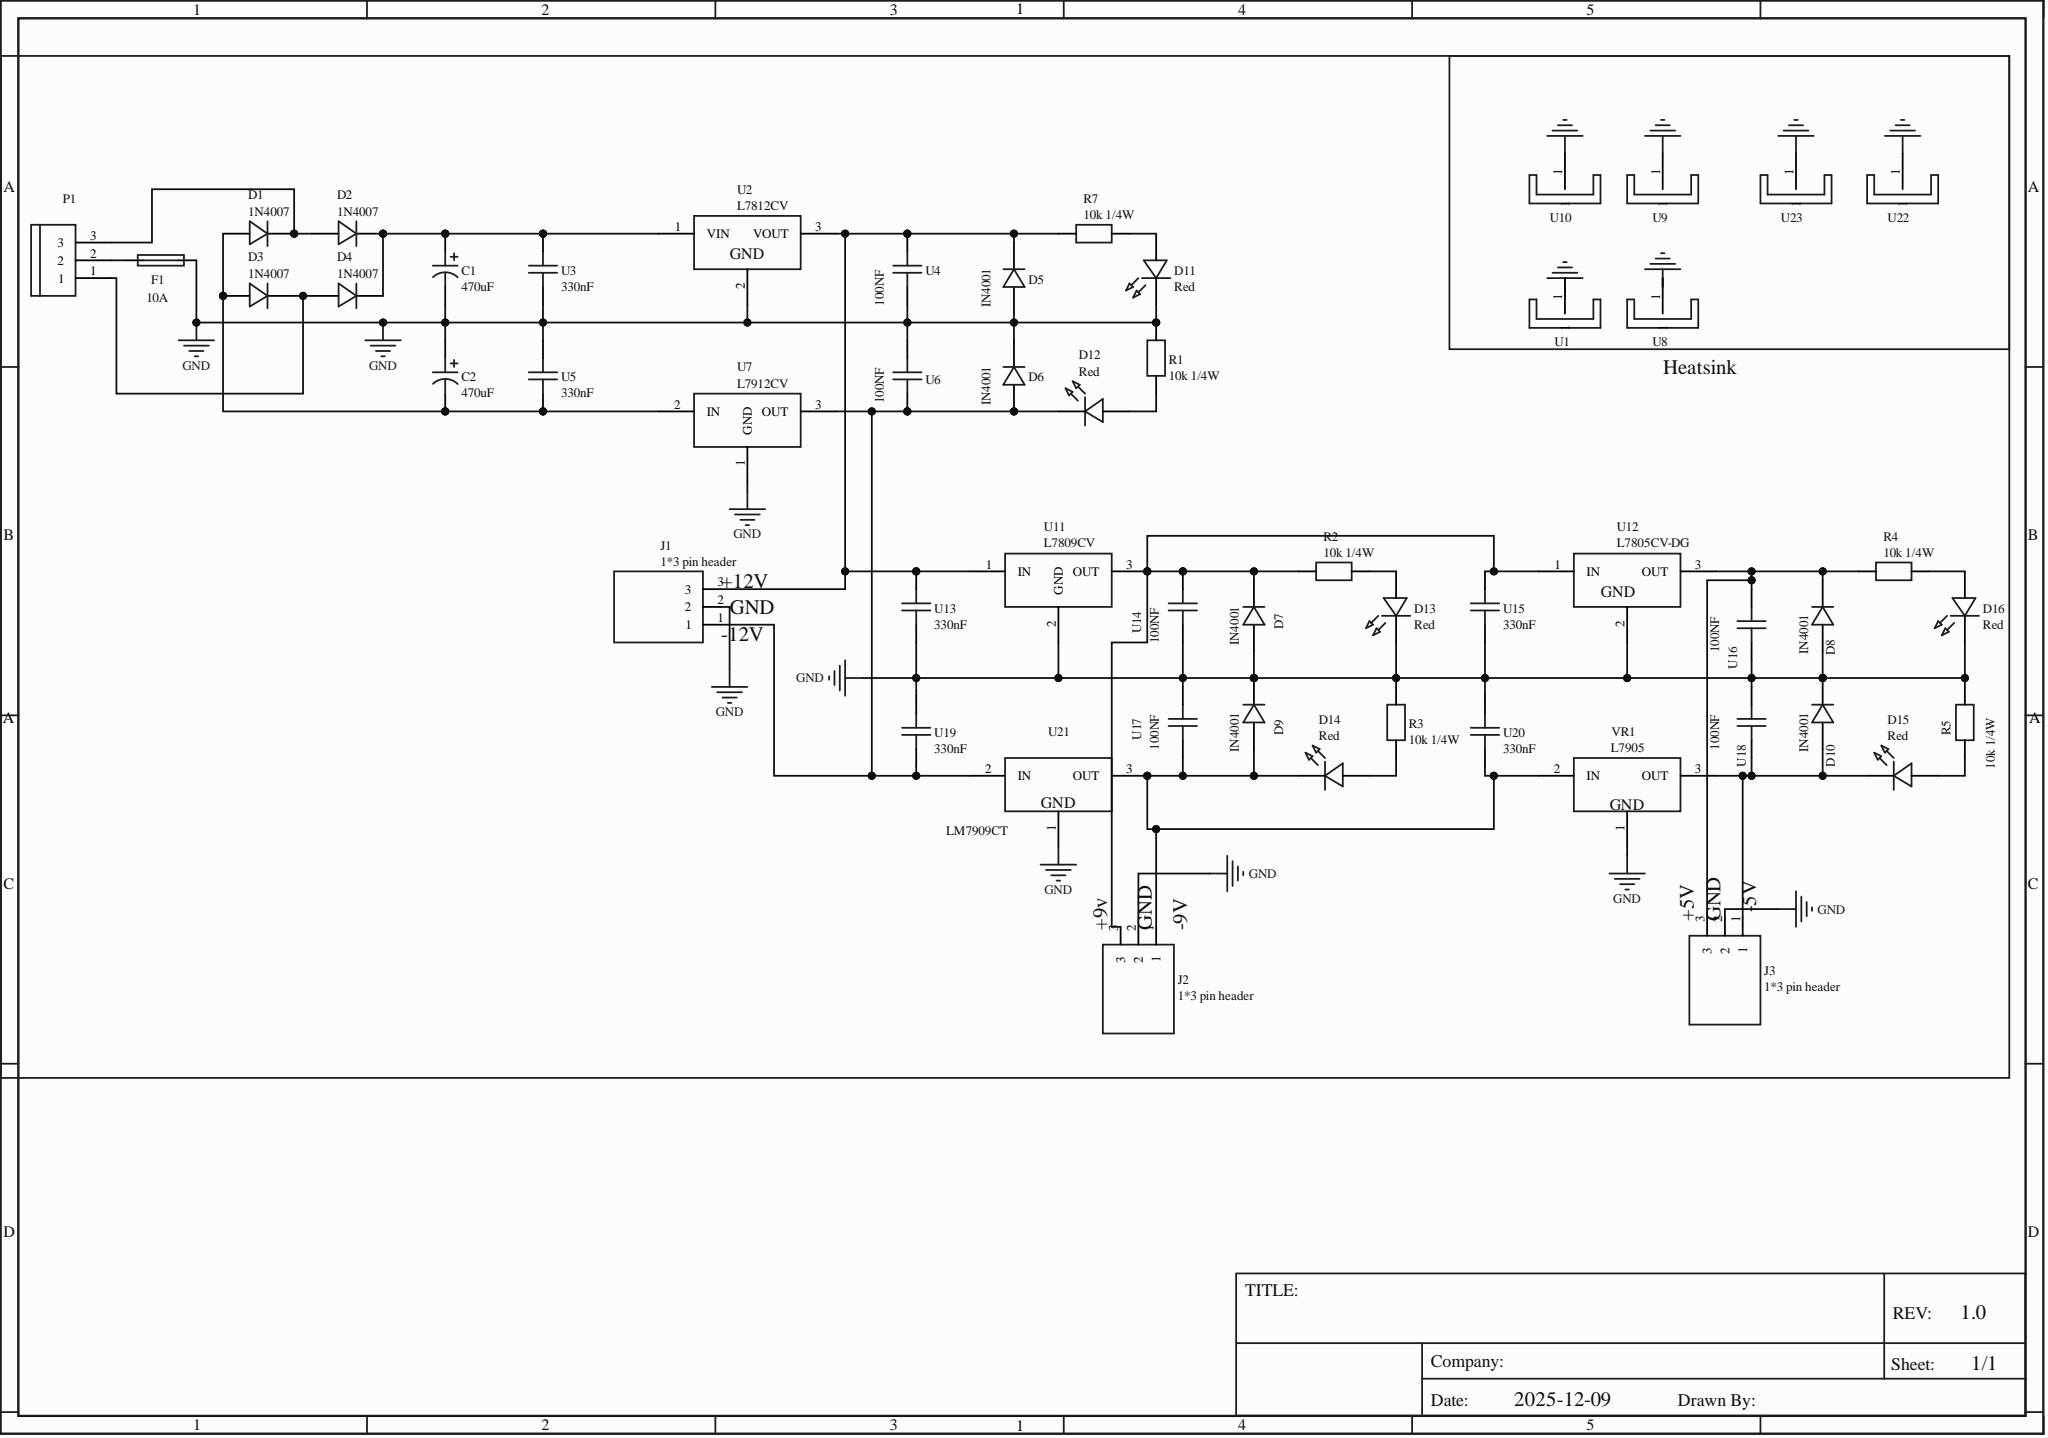Circuit board | Altium Designer | 53 parts | 18 nets
Bill of materials:
Comment,Description,Designator,Footprint,LibRef,Quantity
"470uF","","C1, C2","CAP-TH_BD10.0-P5.00-D0.6-FD","470uF","2"
"1N4007","","D1, D2, D3, D4","DO-41_BD2.4-L4.7-P8.70-D0.9-RD","1N4007","4"
"IN4001","","D5, D6, D7, D8, D9, D10","DO-41_BD2.4-L4.7-P8.70-D0.9-RD","IN4001","6"
"Red","","D11, D12, D13, D14, D15, D16","发光二极管","Red","6"
"10A","","F1","FUSE-SMD_5-20MM","10A","1"
"1*3 pin header","","J1, J2, J3","1*3排针","1*3排针","3"
"WJ500V-5.08-3P","","P1","CONN-TH_3P-P5.00_WJ500V-5.08-3P","WJ500V-5.08-3P","1"
"10k 1/4W","","R1, R2, R3, R4, R5, R7","10K直插电阻 PCB封装","10k 1/4W","6"
"15*10.5*21","","U1, U8, U9, U10, U22, U23","SINK-TH_L15.0-W10.5-H21.0","15*10.5*21","6"
"L7812CV","","U2","TO-220-3_L10.0-W4.5-P2.54-T","L7812CV","1"
"330nF","","U3, U5, U13, U15, U19, U20","CAP-TH_L10.0-W4.0-P7.50-D0.6-1","330nF","6"
"100NF","","U4, U6, U14, U16, U17, U18","CAP-TH_L5.0-W2.5-P5.00-D1.0","100NF","6"
"L7912CV","","U7","TO-220-3_L10.0-W4.5-P2.54-L","L7912CV","1"
"L7809CV","","U11","TO-220-3_L10.0-W4.5-P2.54-L","L7809CV","1"
"L7805CV-DG","","U12","TO-220-3_L10.0-W4.5-P2.54-L","L7805CV-DG","1"
"LM7909CT","","U21","TO-220-3_L10.0-W4.5-P2.54-L","LM7909CT","1"
"L7905","","VR1","TO-220-3_L10.0-W4.5-P2.54-L","L7905","1"
Netlist (Protel format):
[
C1
CAP-TH_BD10.0-P5.00-D0.6-FD
470uF



]
[
C2
CAP-TH_BD10.0-P5.00-D0.6-FD
470uF



]
[
D1
DO-41_BD2.4-L4.7-P8.70-D0.9-RD
1N4007



]
[
D2
DO-41_BD2.4-L4.7-P8.70-D0.9-RD
1N4007



]
[
D3
DO-41_BD2.4-L4.7-P8.70-D0.9-RD
1N4007



]
[
D4
DO-41_BD2.4-L4.7-P8.70-D0.9-RD
1N4007



]
[
D5
DO-41_BD2.4-L4.7-P8.70-D0.9-RD
IN4001



]
[
D6
DO-41_BD2.4-L4.7-P8.70-D0.9-RD
IN4001



]
[
D7
DO-41_BD2.4-L4.7-P8.70-D0.9-RD
IN4001



]
[
D8
DO-41_BD2.4-L4.7-P8.70-D0.9-RD
IN4001



]
[
D9
DO-41_BD2.4-L4.7-P8.70-D0.9-RD
IN4001



]
[
D10
DO-41_BD2.4-L4.7-P8.70-D0.9-RD
IN4001



]
[
D11
发光二极管
Red



]
[
D12
发光二极管
Red



]
[
D13
发光二极管
Red



]
[
D14
发光二极管
Red



]
[
D15
发光二极管
Red



]
[
D16
发光二极管
Red



]
[
F1
FUSE-SMD_5-20MM
10A



]
[
J1
1*3排针
1*3 pin header



]
[
J2
1*3排针
1*3 pin header



]
[
J3
1*3排针
1*3 pin header



]
[
P1
CONN-TH_3P-P5.00_WJ500V-5.08-3P
WJ500V-5.08-3P



]
[
R1
10K直插电阻 PCB封装
10k 1/4W



]
[
R2
10K直插电阻 PCB封装
10k 1/4W



]
[
R3
10K直插电阻 PCB封装
10k 1/4W



]
[
R4
10K直插电阻 PCB封装
10k 1/4W



]
[
R5
10K直插电阻 PCB封装
10k 1/4W



]
[
R7
10K直插电阻 PCB封装
10k 1/4W



]
[
U1
SINK-TH_L15.0-W10.5-H21.0
15*10.5*21



]
[
U2
TO-220-3_L10.0-W4.5-P2.54-T
L7812CV



]
[
U3
CAP-TH_L10.0-W4.0-P7.50-D0.6-1
330nF



]
[
U4
CAP-TH_L5.0-W2.5-P5.00-D1.0
100NF



]
[
U5
CAP-TH_L10.0-W4.0-P7.50-D0.6-1
330nF



]
[
U6
CAP-TH_L5.0-W2.5-P5.00-D1.0
100NF



]
[
U7
TO-220-3_L10.0-W4.5-P2.54-L
L7912CV



]
[
U8
SINK-TH_L15.0-W10.5-H21.0
15*10.5*21



]
[
U9
SINK-TH_L15.0-W10.5-H21.0
15*10.5*21



]
[
U10
SINK-TH_L15.0-W10.5-H21.0
15*10.5*21



]
[
U11
TO-220-3_L10.0-W4.5-P2.54-L
L7809CV



]
[
U12
TO-220-3_L10.0-W4.5-P2.54-L
L7805CV-DG



]
[
U13
CAP-TH_L10.0-W4.0-P7.50-D0.6-1
330nF



]
[
U14
CAP-TH_L5.0-W2.5-P5.00-D1.0
100NF



]
[
U15
CAP-TH_L10.0-W4.0-P7.50-D0.6-1
330nF



]
[
U16
CAP-TH_L5.0-W2.5-P5.00-D1.0
100NF



]
[
U17
CAP-TH_L5.0-W2.5-P5.00-D1.0
100NF



]
[
U18
CAP-TH_L5.0-W2.5-P5.00-D1.0
100NF



]
[
U19
CAP-TH_L10.0-W4.0-P7.50-D0.6-1
330nF



]
[
U20
CAP-TH_L10.0-W4.0-P7.50-D0.6-1
330nF



]
[
U21
TO-220-3_L10.0-W4.5-P2.54-L
LM7909CT



]
[
U22
SINK-TH_L15.0-W10.5-H21.0
15*10.5*21



]
[
U23
SINK-TH_L15.0-W10.5-H21.0
15*10.5*21



]
[
VR1
TO-220-3_L10.0-W4.5-P2.54-L
L7905



]
(
NetF1_1
F1-1
P1-2
)
(
NetD16_1
D16-1
R4-2
)
(
NetD15_1
D15-1
R5-1
)
(
NetD14_1
D14-1
R3-1
)
(
NetD13_1
D13-1
R2-2
)
(
NetD12_1
D12-1
R1-1
)
(
NetD11_1
D11-1
R7-2
)
(
NetD10_2
D10-2
D15-2
J3-1
U18-2
VR1-3
)
(
NetD9_2
D9-2
D14-2
J2-1
U17-2
U20-1
U21-3
VR1-2
)
(
NetD8_1
D8-1
J3-3
R4-1
U12-3
U16-1
)
(
NetD7_1
D7-1
J2-3
R2-1
U11-3
U12-1
U14-1
U15-2
)
(
NetD6_2
D6-2
D12-2
J1-1
U6-2
U7-3
U19-1
U21-2
)
(
NetD5_1
D5-1
J1-3
R7-1
U2-3
U4-1
U11-1
U13-2
)
(
NetD3_1
D3-1
D4-2
P1-1
)
(
NetD1_1
D1-1
D2-2
P1-3
)
(
NetC2_2
C2-2
D1-2
D3-2
U5-1
U7-2
)
(
NetC1_1
C1-1
D2-1
D4-1
U2-1
U3-2
)
(
GND
C1-2
C2-1
D5-2
D6-1
D7-2
D8-2
D9-1
D10-1
D11-2
D13-2
D16-2
F1-2
J1-2
J2-2
J3-2
R1-2
R3-2
R5-2
U1-1
U2-2
U3-1
U4-2
U5-2
U6-1
U7-1
U8-1
U9-1
U10-1
U11-2
U12-2
U13-1
U14-2
U15-1
U16-2
U17-1
U18-1
U19-2
U20-2
U21-1
U22-1
U23-1
VR1-1
)